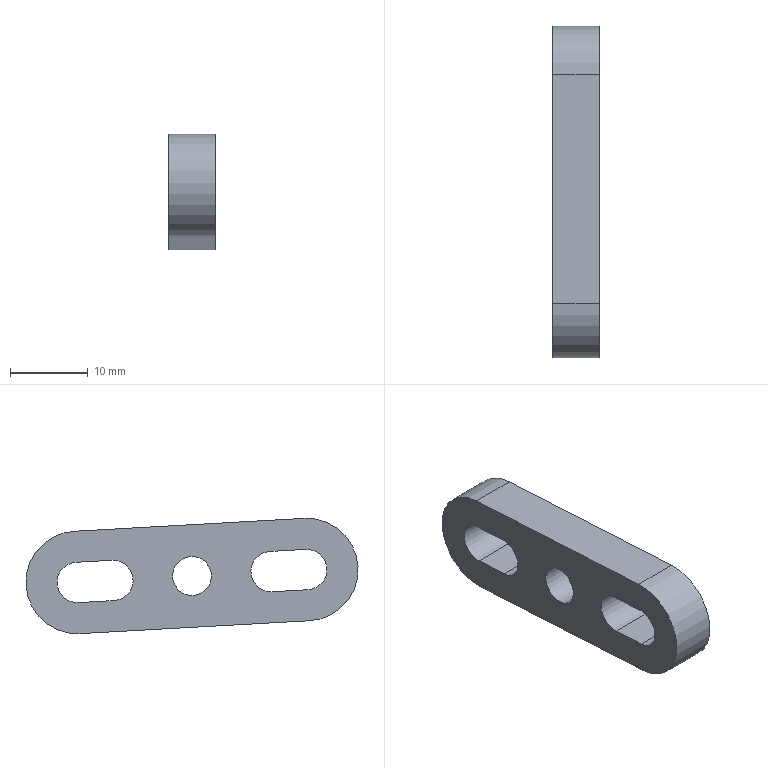Part | STEP file | 1 solid | 15 faces | box 6 x 42.771 x 14.853 mm | volume 2506 mm3 | plane 8 | cylinder 7 | commonest cylinder face diameters 5.2 x4 13.2 x2 5.01 x1
STEP:
#1=CARTESIAN_POINT('',(0.,0.,0.));
#2=DIRECTION('',(0.,0.,1.));
#3=DIRECTION('',(1.,0.,0.));
#4=AXIS2_PLACEMENT_3D('',#1,#2,#3);
#5=CARTESIAN_POINT('',(1826.907,485.05,14.25));
#6=VERTEX_POINT('',#5);
#7=CARTESIAN_POINT('',(1826.907,489.66,13.992));
#8=VERTEX_POINT('',#7);
#9=CARTESIAN_POINT('',(1826.907,489.66,13.992));
#10=DIRECTION('',(0.,0.9984,-0.05582));
#11=VECTOR('',#10,1.);
#12=LINE('',#9,#11);
#13=CARTESIAN_POINT('',(1832.907,489.66,13.992));
#14=DIRECTION('',(0.,0.05582,0.9984));
#15=DIRECTION('',(1.,0.,0.));
#16=AXIS2_PLACEMENT_3D('',#13,#14,#15);
#17=PLANE('',#16);
#18=CARTESIAN_POINT('',(-6.,0.));
#19=DIRECTION('',(0.,1.));
#20=VECTOR('',#19,1.);
#21=LINE('',#18,#20);
#22=(GEOMETRIC_REPRESENTATION_CONTEXT(2)PARAMETRIC_REPRESENTATION_CONTEXT()REPRESENTATION_CONTEXT('',''));
#23=DEFINITIONAL_REPRESENTATION('',(#21),#22);
#24=PCURVE('',#17,#23);
#25=CARTESIAN_POINT('',(1826.907,485.195,16.846));
#26=DIRECTION('',(-1.,0.,0.));
#27=DIRECTION('',(0.,0.05582,0.9984));
#28=AXIS2_PLACEMENT_3D('',#25,#26,#27);
#29=PLANE('',#28);
#30=CARTESIAN_POINT('',(-2.6,4.618));
#31=DIRECTION('',(0.,1.));
#32=VECTOR('',#31,1.);
#33=LINE('',#30,#32);
#34=(GEOMETRIC_REPRESENTATION_CONTEXT(2)PARAMETRIC_REPRESENTATION_CONTEXT()REPRESENTATION_CONTEXT('',''));
#35=DEFINITIONAL_REPRESENTATION('',(#33),#34);
#36=PCURVE('',#29,#35);
#37=SURFACE_CURVE('',#12,(#24,#36),.PCURVE_S1.);
#38=EDGE_CURVE('',#6,#8,#37,.T.);
#39=ORIENTED_EDGE('',*,*,#38,.F.);
#40=CARTESIAN_POINT('',(1832.907,485.05,14.25));
#41=VERTEX_POINT('',#40);
#42=CARTESIAN_POINT('',(1832.907,485.05,14.25));
#43=DIRECTION('',(1.,0.,0.));
#44=VECTOR('',#43,1.);
#45=LINE('',#42,#44);
#46=CARTESIAN_POINT('',(0.,-4.618));
#47=DIRECTION('',(1.,0.));
#48=VECTOR('',#47,1.);
#49=LINE('',#46,#48);
#50=(GEOMETRIC_REPRESENTATION_CONTEXT(2)PARAMETRIC_REPRESENTATION_CONTEXT()REPRESENTATION_CONTEXT('',''));
#51=DEFINITIONAL_REPRESENTATION('',(#49),#50);
#52=PCURVE('',#17,#51);
#53=CARTESIAN_POINT('',(1832.907,485.195,16.846));
#54=DIRECTION('',(-1.,0.,0.));
#55=DIRECTION('',(0.,0.05582,0.9984));
#56=AXIS2_PLACEMENT_3D('',#53,#54,#55);
#57=CYLINDRICAL_SURFACE('',#56,2.6);
#58=CARTESIAN_POINT('',(3.142,0.));
#59=DIRECTION('',(0.,-1.));
#60=VECTOR('',#59,1.);
#61=LINE('',#58,#60);
#62=(GEOMETRIC_REPRESENTATION_CONTEXT(2)PARAMETRIC_REPRESENTATION_CONTEXT()REPRESENTATION_CONTEXT('',''));
#63=DEFINITIONAL_REPRESENTATION('',(#61),#62);
#64=PCURVE('',#57,#63);
#65=SURFACE_CURVE('',#45,(#52,#64),.PCURVE_S1.);
#66=EDGE_CURVE('',#6,#41,#65,.T.);
#67=ORIENTED_EDGE('',*,*,#66,.T.);
#68=CARTESIAN_POINT('',(1832.907,489.66,13.992));
#69=VERTEX_POINT('',#68);
#70=CARTESIAN_POINT('',(1832.907,489.66,13.992));
#71=DIRECTION('',(0.,0.9984,-0.05582));
#72=VECTOR('',#71,1.);
#73=LINE('',#70,#72);
#74=CARTESIAN_POINT('',(0.,0.));
#75=DIRECTION('',(0.,1.));
#76=VECTOR('',#75,1.);
#77=LINE('',#74,#76);
#78=(GEOMETRIC_REPRESENTATION_CONTEXT(2)PARAMETRIC_REPRESENTATION_CONTEXT()REPRESENTATION_CONTEXT('',''));
#79=DEFINITIONAL_REPRESENTATION('',(#77),#78);
#80=PCURVE('',#17,#79);
#81=CARTESIAN_POINT('',(1832.907,485.195,16.846));
#82=DIRECTION('',(-1.,0.,0.));
#83=DIRECTION('',(0.,0.05582,0.9984));
#84=AXIS2_PLACEMENT_3D('',#81,#82,#83);
#85=PLANE('',#84);
#86=CARTESIAN_POINT('',(-2.6,4.618));
#87=DIRECTION('',(0.,1.));
#88=VECTOR('',#87,1.);
#89=LINE('',#86,#88);
#90=(GEOMETRIC_REPRESENTATION_CONTEXT(2)PARAMETRIC_REPRESENTATION_CONTEXT()REPRESENTATION_CONTEXT('',''));
#91=DEFINITIONAL_REPRESENTATION('',(#89),#90);
#92=PCURVE('',#85,#91);
#93=SURFACE_CURVE('',#73,(#80,#92),.PCURVE_S1.);
#94=EDGE_CURVE('',#41,#69,#93,.T.);
#95=ORIENTED_EDGE('',*,*,#94,.T.);
#96=CARTESIAN_POINT('',(1832.907,489.66,13.992));
#97=DIRECTION('',(1.,0.,0.));
#98=VECTOR('',#97,1.);
#99=LINE('',#96,#98);
#100=CARTESIAN_POINT('',(0.,0.));
#101=DIRECTION('',(1.,0.));
#102=VECTOR('',#101,1.);
#103=LINE('',#100,#102);
#104=(GEOMETRIC_REPRESENTATION_CONTEXT(2)PARAMETRIC_REPRESENTATION_CONTEXT()REPRESENTATION_CONTEXT('',''));
#105=DEFINITIONAL_REPRESENTATION('',(#103),#104);
#106=PCURVE('',#17,#105);
#107=CARTESIAN_POINT('',(1832.907,489.805,16.588));
#108=DIRECTION('',(-1.,0.,0.));
#109=DIRECTION('',(0.,0.05582,0.9984));
#110=AXIS2_PLACEMENT_3D('',#107,#108,#109);
#111=CYLINDRICAL_SURFACE('',#110,2.6);
#112=CARTESIAN_POINT('',(3.142,0.));
#113=DIRECTION('',(0.,-1.));
#114=VECTOR('',#113,1.);
#115=LINE('',#112,#114);
#116=(GEOMETRIC_REPRESENTATION_CONTEXT(2)PARAMETRIC_REPRESENTATION_CONTEXT()REPRESENTATION_CONTEXT('',''));
#117=DEFINITIONAL_REPRESENTATION('',(#115),#116);
#118=PCURVE('',#111,#117);
#119=SURFACE_CURVE('',#99,(#106,#118),.PCURVE_S1.);
#120=EDGE_CURVE('',#8,#69,#119,.T.);
#121=ORIENTED_EDGE('',*,*,#120,.F.);
#122=EDGE_LOOP('',(#39,#67,#95,#121));
#123=FACE_BOUND('',#122,.T.);
#124=ADVANCED_FACE('',(#123),#17,.T.);
#125=ORIENTED_EDGE('',*,*,#66,.T.);
#126=CARTESIAN_POINT('',(1832.907,485.34,19.442));
#127=VERTEX_POINT('',#126);
#128=CARTESIAN_POINT('',(1832.907,485.195,16.846));
#129=DIRECTION('',(1.,0.,0.));
#130=DIRECTION('',(0.,0.05582,0.9984));
#131=AXIS2_PLACEMENT_3D('',#128,#129,#130);
#132=CIRCLE('',#131,2.6);
#133=CARTESIAN_POINT('',(6.283,0.));
#134=DIRECTION('',(-1.,0.));
#135=VECTOR('',#134,1.);
#136=LINE('',#133,#135);
#137=(GEOMETRIC_REPRESENTATION_CONTEXT(2)PARAMETRIC_REPRESENTATION_CONTEXT()REPRESENTATION_CONTEXT('',''));
#138=DEFINITIONAL_REPRESENTATION('',(#136),#137);
#139=PCURVE('',#57,#138);
#140=CARTESIAN_POINT('',(2.6,0.));
#141=CARTESIAN_POINT('',(2.6,-4.503));
#142=CARTESIAN_POINT('',(-1.3,-2.252));
#143=CARTESIAN_POINT('',(-5.2,0.));
#144=CARTESIAN_POINT('',(-1.3,2.252));
#145=CARTESIAN_POINT('',(2.6,4.503));
#146=CARTESIAN_POINT('',(2.6,0.));
#147=(BOUNDED_CURVE()B_SPLINE_CURVE(2,(#140,#141,#142,#143,#144,#145,#146),.UNSPECIFIED.,.T.,.F.)B_SPLINE_CURVE_WITH_KNOTS((1,2,2,2,2,1),(-2.094,0.,2.094,4.189,6.283,8.378),.UNSPECIFIED.)CURVE()GEOMETRIC_REPRESENTATION_ITEM()RATIONAL_B_SPLINE_CURVE((1.,0.5,1.,0.5,1.,0.5,1.))REPRESENTATION_ITEM(''));
#148=(GEOMETRIC_REPRESENTATION_CONTEXT(2)PARAMETRIC_REPRESENTATION_CONTEXT()REPRESENTATION_CONTEXT('',''));
#149=DEFINITIONAL_REPRESENTATION('',(#147),#148);
#150=PCURVE('',#85,#149);
#151=SURFACE_CURVE('',#132,(#139,#150),.PCURVE_S1.);
#152=EDGE_CURVE('',#127,#41,#151,.T.);
#153=ORIENTED_EDGE('',*,*,#152,.F.);
#154=CARTESIAN_POINT('',(1826.907,485.34,19.442));
#155=VERTEX_POINT('',#154);
#156=CARTESIAN_POINT('',(1832.907,485.34,19.442));
#157=DIRECTION('',(1.,0.,0.));
#158=VECTOR('',#157,1.);
#159=LINE('',#156,#158);
#160=CARTESIAN_POINT('',(6.283,0.));
#161=DIRECTION('',(0.,-1.));
#162=VECTOR('',#161,1.);
#163=LINE('',#160,#162);
#164=(GEOMETRIC_REPRESENTATION_CONTEXT(2)PARAMETRIC_REPRESENTATION_CONTEXT()REPRESENTATION_CONTEXT('',''));
#165=DEFINITIONAL_REPRESENTATION('',(#163),#164);
#166=PCURVE('',#57,#165);
#167=CARTESIAN_POINT('',(1832.907,485.34,19.442));
#168=DIRECTION('',(0.,-0.05582,-0.9984));
#169=DIRECTION('',(-1.,0.,0.));
#170=AXIS2_PLACEMENT_3D('',#167,#168,#169);
#171=PLANE('',#170);
#172=CARTESIAN_POINT('',(0.,0.));
#173=DIRECTION('',(-1.,0.));
#174=VECTOR('',#173,1.);
#175=LINE('',#172,#174);
#176=(GEOMETRIC_REPRESENTATION_CONTEXT(2)PARAMETRIC_REPRESENTATION_CONTEXT()REPRESENTATION_CONTEXT('',''));
#177=DEFINITIONAL_REPRESENTATION('',(#175),#176);
#178=PCURVE('',#171,#177);
#179=SURFACE_CURVE('',#159,(#166,#178),.PCURVE_S1.);
#180=EDGE_CURVE('',#155,#127,#179,.T.);
#181=ORIENTED_EDGE('',*,*,#180,.F.);
#182=CARTESIAN_POINT('',(1826.907,485.195,16.846));
#183=DIRECTION('',(1.,0.,0.));
#184=DIRECTION('',(0.,0.05582,0.9984));
#185=AXIS2_PLACEMENT_3D('',#182,#183,#184);
#186=CIRCLE('',#185,2.6);
#187=CARTESIAN_POINT('',(6.283,6.));
#188=DIRECTION('',(-1.,0.));
#189=VECTOR('',#188,1.);
#190=LINE('',#187,#189);
#191=(GEOMETRIC_REPRESENTATION_CONTEXT(2)PARAMETRIC_REPRESENTATION_CONTEXT()REPRESENTATION_CONTEXT('',''));
#192=DEFINITIONAL_REPRESENTATION('',(#190),#191);
#193=PCURVE('',#57,#192);
#194=CARTESIAN_POINT('',(2.6,0.));
#195=CARTESIAN_POINT('',(2.6,-4.503));
#196=CARTESIAN_POINT('',(-1.3,-2.252));
#197=CARTESIAN_POINT('',(-5.2,0.));
#198=CARTESIAN_POINT('',(-1.3,2.252));
#199=CARTESIAN_POINT('',(2.6,4.503));
#200=CARTESIAN_POINT('',(2.6,0.));
#201=(BOUNDED_CURVE()B_SPLINE_CURVE(2,(#194,#195,#196,#197,#198,#199,#200),.UNSPECIFIED.,.T.,.F.)B_SPLINE_CURVE_WITH_KNOTS((1,2,2,2,2,1),(-2.094,0.,2.094,4.189,6.283,8.378),.UNSPECIFIED.)CURVE()GEOMETRIC_REPRESENTATION_ITEM()RATIONAL_B_SPLINE_CURVE((1.,0.5,1.,0.5,1.,0.5,1.))REPRESENTATION_ITEM(''));
#202=(GEOMETRIC_REPRESENTATION_CONTEXT(2)PARAMETRIC_REPRESENTATION_CONTEXT()REPRESENTATION_CONTEXT('',''));
#203=DEFINITIONAL_REPRESENTATION('',(#201),#202);
#204=PCURVE('',#29,#203);
#205=SURFACE_CURVE('',#186,(#193,#204),.PCURVE_S1.);
#206=EDGE_CURVE('',#155,#6,#205,.T.);
#207=ORIENTED_EDGE('',*,*,#206,.T.);
#208=EDGE_LOOP('',(#125,#153,#181,#207));
#209=FACE_BOUND('',#208,.F.);
#210=ADVANCED_FACE('',(#209),#57,.F.);
#211=CARTESIAN_POINT('',(1826.907,489.95,19.184));
#212=VERTEX_POINT('',#211);
#213=CARTESIAN_POINT('',(1826.907,485.34,19.442));
#214=DIRECTION('',(0.,-0.9984,0.05582));
#215=VECTOR('',#214,1.);
#216=LINE('',#213,#215);
#217=CARTESIAN_POINT('',(6.,0.));
#218=DIRECTION('',(0.,-1.));
#219=VECTOR('',#218,1.);
#220=LINE('',#217,#219);
#221=(GEOMETRIC_REPRESENTATION_CONTEXT(2)PARAMETRIC_REPRESENTATION_CONTEXT()REPRESENTATION_CONTEXT('',''));
#222=DEFINITIONAL_REPRESENTATION('',(#220),#221);
#223=PCURVE('',#171,#222);
#224=CARTESIAN_POINT('',(2.6,0.));
#225=DIRECTION('',(0.,-1.));
#226=VECTOR('',#225,1.);
#227=LINE('',#224,#226);
#228=(GEOMETRIC_REPRESENTATION_CONTEXT(2)PARAMETRIC_REPRESENTATION_CONTEXT()REPRESENTATION_CONTEXT('',''));
#229=DEFINITIONAL_REPRESENTATION('',(#227),#228);
#230=PCURVE('',#29,#229);
#231=SURFACE_CURVE('',#216,(#223,#230),.PCURVE_S1.);
#232=EDGE_CURVE('',#212,#155,#231,.T.);
#233=ORIENTED_EDGE('',*,*,#232,.F.);
#234=CARTESIAN_POINT('',(1832.907,489.95,19.184));
#235=VERTEX_POINT('',#234);
#236=CARTESIAN_POINT('',(1832.907,489.95,19.184));
#237=DIRECTION('',(1.,0.,0.));
#238=VECTOR('',#237,1.);
#239=LINE('',#236,#238);
#240=CARTESIAN_POINT('',(0.,4.618));
#241=DIRECTION('',(-1.,0.));
#242=VECTOR('',#241,1.);
#243=LINE('',#240,#242);
#244=(GEOMETRIC_REPRESENTATION_CONTEXT(2)PARAMETRIC_REPRESENTATION_CONTEXT()REPRESENTATION_CONTEXT('',''));
#245=DEFINITIONAL_REPRESENTATION('',(#243),#244);
#246=PCURVE('',#171,#245);
#247=CARTESIAN_POINT('',(0.,0.));
#248=DIRECTION('',(0.,-1.));
#249=VECTOR('',#248,1.);
#250=LINE('',#247,#249);
#251=(GEOMETRIC_REPRESENTATION_CONTEXT(2)PARAMETRIC_REPRESENTATION_CONTEXT()REPRESENTATION_CONTEXT('',''));
#252=DEFINITIONAL_REPRESENTATION('',(#250),#251);
#253=PCURVE('',#111,#252);
#254=SURFACE_CURVE('',#239,(#246,#253),.PCURVE_S1.);
#255=EDGE_CURVE('',#212,#235,#254,.T.);
#256=ORIENTED_EDGE('',*,*,#255,.T.);
#257=CARTESIAN_POINT('',(1832.907,485.34,19.442));
#258=DIRECTION('',(0.,-0.9984,0.05582));
#259=VECTOR('',#258,1.);
#260=LINE('',#257,#259);
#261=CARTESIAN_POINT('',(0.,0.));
#262=DIRECTION('',(0.,-1.));
#263=VECTOR('',#262,1.);
#264=LINE('',#261,#263);
#265=(GEOMETRIC_REPRESENTATION_CONTEXT(2)PARAMETRIC_REPRESENTATION_CONTEXT()REPRESENTATION_CONTEXT('',''));
#266=DEFINITIONAL_REPRESENTATION('',(#264),#265);
#267=PCURVE('',#171,#266);
#268=CARTESIAN_POINT('',(2.6,0.));
#269=DIRECTION('',(0.,-1.));
#270=VECTOR('',#269,1.);
#271=LINE('',#268,#270);
#272=(GEOMETRIC_REPRESENTATION_CONTEXT(2)PARAMETRIC_REPRESENTATION_CONTEXT()REPRESENTATION_CONTEXT('',''));
#273=DEFINITIONAL_REPRESENTATION('',(#271),#272);
#274=PCURVE('',#85,#273);
#275=SURFACE_CURVE('',#260,(#267,#274),.PCURVE_S1.);
#276=EDGE_CURVE('',#235,#127,#275,.T.);
#277=ORIENTED_EDGE('',*,*,#276,.T.);
#278=ORIENTED_EDGE('',*,*,#180,.F.);
#279=EDGE_LOOP('',(#233,#256,#277,#278));
#280=FACE_BOUND('',#279,.T.);
#281=ADVANCED_FACE('',(#280),#171,.T.);
#282=CARTESIAN_POINT('',(1826.907,510.01,12.854));
#283=VERTEX_POINT('',#282);
#284=CARTESIAN_POINT('',(1826.907,514.621,12.597));
#285=VERTEX_POINT('',#284);
#286=CARTESIAN_POINT('',(1826.907,514.621,12.597));
#287=DIRECTION('',(0.,0.9984,-0.05582));
#288=VECTOR('',#287,1.);
#289=LINE('',#286,#288);
#290=CARTESIAN_POINT('',(1832.907,514.621,12.597));
#291=DIRECTION('',(0.,0.05582,0.9984));
#292=DIRECTION('',(0.,-0.9984,0.05582));
#293=AXIS2_PLACEMENT_3D('',#290,#291,#292);
#294=PLANE('',#293);
#295=CARTESIAN_POINT('',(0.,-6.));
#296=DIRECTION('',(-1.,0.));
#297=VECTOR('',#296,1.);
#298=LINE('',#295,#297);
#299=(GEOMETRIC_REPRESENTATION_CONTEXT(2)PARAMETRIC_REPRESENTATION_CONTEXT()REPRESENTATION_CONTEXT('',''));
#300=DEFINITIONAL_REPRESENTATION('',(#298),#299);
#301=PCURVE('',#294,#300);
#302=CARTESIAN_POINT('',(-2.6,29.617));
#303=DIRECTION('',(0.,1.));
#304=VECTOR('',#303,1.);
#305=LINE('',#302,#304);
#306=(GEOMETRIC_REPRESENTATION_CONTEXT(2)PARAMETRIC_REPRESENTATION_CONTEXT()REPRESENTATION_CONTEXT('',''));
#307=DEFINITIONAL_REPRESENTATION('',(#305),#306);
#308=PCURVE('',#29,#307);
#309=SURFACE_CURVE('',#289,(#301,#308),.PCURVE_S1.);
#310=EDGE_CURVE('',#283,#285,#309,.T.);
#311=ORIENTED_EDGE('',*,*,#310,.F.);
#312=CARTESIAN_POINT('',(1832.907,510.01,12.854));
#313=VERTEX_POINT('',#312);
#314=CARTESIAN_POINT('',(1832.907,510.01,12.854));
#315=DIRECTION('',(1.,0.,0.));
#316=VECTOR('',#315,1.);
#317=LINE('',#314,#316);
#318=CARTESIAN_POINT('',(4.618,0.));
#319=DIRECTION('',(0.,1.));
#320=VECTOR('',#319,1.);
#321=LINE('',#318,#320);
#322=(GEOMETRIC_REPRESENTATION_CONTEXT(2)PARAMETRIC_REPRESENTATION_CONTEXT()REPRESENTATION_CONTEXT('',''));
#323=DEFINITIONAL_REPRESENTATION('',(#321),#322);
#324=PCURVE('',#294,#323);
#325=CARTESIAN_POINT('',(1832.907,510.156,15.45));
#326=DIRECTION('',(-1.,0.,0.));
#327=DIRECTION('',(0.,0.05582,0.9984));
#328=AXIS2_PLACEMENT_3D('',#325,#326,#327);
#329=CYLINDRICAL_SURFACE('',#328,2.6);
#330=CARTESIAN_POINT('',(3.142,0.));
#331=DIRECTION('',(0.,-1.));
#332=VECTOR('',#331,1.);
#333=LINE('',#330,#332);
#334=(GEOMETRIC_REPRESENTATION_CONTEXT(2)PARAMETRIC_REPRESENTATION_CONTEXT()REPRESENTATION_CONTEXT('',''));
#335=DEFINITIONAL_REPRESENTATION('',(#333),#334);
#336=PCURVE('',#329,#335);
#337=SURFACE_CURVE('',#317,(#324,#336),.PCURVE_S1.);
#338=EDGE_CURVE('',#283,#313,#337,.T.);
#339=ORIENTED_EDGE('',*,*,#338,.T.);
#340=CARTESIAN_POINT('',(1832.907,514.621,12.597));
#341=VERTEX_POINT('',#340);
#342=CARTESIAN_POINT('',(1832.907,514.621,12.597));
#343=DIRECTION('',(0.,0.9984,-0.05582));
#344=VECTOR('',#343,1.);
#345=LINE('',#342,#344);
#346=CARTESIAN_POINT('',(0.,0.));
#347=DIRECTION('',(-1.,0.));
#348=VECTOR('',#347,1.);
#349=LINE('',#346,#348);
#350=(GEOMETRIC_REPRESENTATION_CONTEXT(2)PARAMETRIC_REPRESENTATION_CONTEXT()REPRESENTATION_CONTEXT('',''));
#351=DEFINITIONAL_REPRESENTATION('',(#349),#350);
#352=PCURVE('',#294,#351);
#353=CARTESIAN_POINT('',(-2.6,29.617));
#354=DIRECTION('',(0.,1.));
#355=VECTOR('',#354,1.);
#356=LINE('',#353,#355);
#357=(GEOMETRIC_REPRESENTATION_CONTEXT(2)PARAMETRIC_REPRESENTATION_CONTEXT()REPRESENTATION_CONTEXT('',''));
#358=DEFINITIONAL_REPRESENTATION('',(#356),#357);
#359=PCURVE('',#85,#358);
#360=SURFACE_CURVE('',#345,(#352,#359),.PCURVE_S1.);
#361=EDGE_CURVE('',#313,#341,#360,.T.);
#362=ORIENTED_EDGE('',*,*,#361,.T.);
#363=CARTESIAN_POINT('',(1832.907,514.621,12.597));
#364=DIRECTION('',(1.,0.,0.));
#365=VECTOR('',#364,1.);
#366=LINE('',#363,#365);
#367=CARTESIAN_POINT('',(0.,0.));
#368=DIRECTION('',(0.,1.));
#369=VECTOR('',#368,1.);
#370=LINE('',#367,#369);
#371=(GEOMETRIC_REPRESENTATION_CONTEXT(2)PARAMETRIC_REPRESENTATION_CONTEXT()REPRESENTATION_CONTEXT('',''));
#372=DEFINITIONAL_REPRESENTATION('',(#370),#371);
#373=PCURVE('',#294,#372);
#374=CARTESIAN_POINT('',(1832.907,514.766,15.192));
#375=DIRECTION('',(-1.,0.,0.));
#376=DIRECTION('',(0.,0.05582,0.9984));
#377=AXIS2_PLACEMENT_3D('',#374,#375,#376);
#378=CYLINDRICAL_SURFACE('',#377,2.6);
#379=CARTESIAN_POINT('',(3.142,0.));
#380=DIRECTION('',(0.,-1.));
#381=VECTOR('',#380,1.);
#382=LINE('',#379,#381);
#383=(GEOMETRIC_REPRESENTATION_CONTEXT(2)PARAMETRIC_REPRESENTATION_CONTEXT()REPRESENTATION_CONTEXT('',''));
#384=DEFINITIONAL_REPRESENTATION('',(#382),#383);
#385=PCURVE('',#378,#384);
#386=SURFACE_CURVE('',#366,(#373,#385),.PCURVE_S1.);
#387=EDGE_CURVE('',#285,#341,#386,.T.);
#388=ORIENTED_EDGE('',*,*,#387,.F.);
#389=EDGE_LOOP('',(#311,#339,#362,#388));
#390=FACE_BOUND('',#389,.T.);
#391=ADVANCED_FACE('',(#390),#294,.T.);
#392=ORIENTED_EDGE('',*,*,#338,.T.);
#393=CARTESIAN_POINT('',(1832.907,510.301,18.046));
#394=VERTEX_POINT('',#393);
#395=CARTESIAN_POINT('',(1832.907,510.156,15.45));
#396=DIRECTION('',(1.,0.,0.));
#397=DIRECTION('',(0.,0.05582,0.9984));
#398=AXIS2_PLACEMENT_3D('',#395,#396,#397);
#399=CIRCLE('',#398,2.6);
#400=CARTESIAN_POINT('',(6.283,0.));
#401=DIRECTION('',(-1.,0.));
#402=VECTOR('',#401,1.);
#403=LINE('',#400,#402);
#404=(GEOMETRIC_REPRESENTATION_CONTEXT(2)PARAMETRIC_REPRESENTATION_CONTEXT()REPRESENTATION_CONTEXT('',''));
#405=DEFINITIONAL_REPRESENTATION('',(#403),#404);
#406=PCURVE('',#329,#405);
#407=CARTESIAN_POINT('',(2.6,25.));
#408=CARTESIAN_POINT('',(2.6,20.496));
#409=CARTESIAN_POINT('',(-1.3,22.748));
#410=CARTESIAN_POINT('',(-5.2,25.));
#411=CARTESIAN_POINT('',(-1.3,27.251));
#412=CARTESIAN_POINT('',(2.6,29.503));
#413=CARTESIAN_POINT('',(2.6,25.));
#414=(BOUNDED_CURVE()B_SPLINE_CURVE(2,(#407,#408,#409,#410,#411,#412,#413),.UNSPECIFIED.,.T.,.F.)B_SPLINE_CURVE_WITH_KNOTS((1,2,2,2,2,1),(-2.094,0.,2.094,4.189,6.283,8.378),.UNSPECIFIED.)CURVE()GEOMETRIC_REPRESENTATION_ITEM()RATIONAL_B_SPLINE_CURVE((1.,0.5,1.,0.5,1.,0.5,1.))REPRESENTATION_ITEM(''));
#415=(GEOMETRIC_REPRESENTATION_CONTEXT(2)PARAMETRIC_REPRESENTATION_CONTEXT()REPRESENTATION_CONTEXT('',''));
#416=DEFINITIONAL_REPRESENTATION('',(#414),#415);
#417=PCURVE('',#85,#416);
#418=SURFACE_CURVE('',#399,(#406,#417),.PCURVE_S1.);
#419=EDGE_CURVE('',#394,#313,#418,.T.);
#420=ORIENTED_EDGE('',*,*,#419,.F.);
#421=CARTESIAN_POINT('',(1826.907,510.301,18.046));
#422=VERTEX_POINT('',#421);
#423=CARTESIAN_POINT('',(1832.907,510.301,18.046));
#424=DIRECTION('',(1.,0.,0.));
#425=VECTOR('',#424,1.);
#426=LINE('',#423,#425);
#427=CARTESIAN_POINT('',(6.283,0.));
#428=DIRECTION('',(0.,-1.));
#429=VECTOR('',#428,1.);
#430=LINE('',#427,#429);
#431=(GEOMETRIC_REPRESENTATION_CONTEXT(2)PARAMETRIC_REPRESENTATION_CONTEXT()REPRESENTATION_CONTEXT('',''));
#432=DEFINITIONAL_REPRESENTATION('',(#430),#431);
#433=PCURVE('',#329,#432);
#434=CARTESIAN_POINT('',(1832.907,510.301,18.046));
#435=DIRECTION('',(0.,-0.05582,-0.9984));
#436=DIRECTION('',(-1.,0.,0.));
#437=AXIS2_PLACEMENT_3D('',#434,#435,#436);
#438=PLANE('',#437);
#439=CARTESIAN_POINT('',(0.,0.));
#440=DIRECTION('',(-1.,0.));
#441=VECTOR('',#440,1.);
#442=LINE('',#439,#441);
#443=(GEOMETRIC_REPRESENTATION_CONTEXT(2)PARAMETRIC_REPRESENTATION_CONTEXT()REPRESENTATION_CONTEXT('',''));
#444=DEFINITIONAL_REPRESENTATION('',(#442),#443);
#445=PCURVE('',#438,#444);
#446=SURFACE_CURVE('',#426,(#433,#445),.PCURVE_S1.);
#447=EDGE_CURVE('',#422,#394,#446,.T.);
#448=ORIENTED_EDGE('',*,*,#447,.F.);
#449=CARTESIAN_POINT('',(1826.907,510.156,15.45));
#450=DIRECTION('',(1.,0.,0.));
#451=DIRECTION('',(0.,0.05582,0.9984));
#452=AXIS2_PLACEMENT_3D('',#449,#450,#451);
#453=CIRCLE('',#452,2.6);
#454=CARTESIAN_POINT('',(6.283,6.));
#455=DIRECTION('',(-1.,0.));
#456=VECTOR('',#455,1.);
#457=LINE('',#454,#456);
#458=(GEOMETRIC_REPRESENTATION_CONTEXT(2)PARAMETRIC_REPRESENTATION_CONTEXT()REPRESENTATION_CONTEXT('',''));
#459=DEFINITIONAL_REPRESENTATION('',(#457),#458);
#460=PCURVE('',#329,#459);
#461=CARTESIAN_POINT('',(2.6,25.));
#462=CARTESIAN_POINT('',(2.6,20.496));
#463=CARTESIAN_POINT('',(-1.3,22.748));
#464=CARTESIAN_POINT('',(-5.2,25.));
#465=CARTESIAN_POINT('',(-1.3,27.251));
#466=CARTESIAN_POINT('',(2.6,29.503));
#467=CARTESIAN_POINT('',(2.6,25.));
#468=(BOUNDED_CURVE()B_SPLINE_CURVE(2,(#461,#462,#463,#464,#465,#466,#467),.UNSPECIFIED.,.T.,.F.)B_SPLINE_CURVE_WITH_KNOTS((1,2,2,2,2,1),(-2.094,0.,2.094,4.189,6.283,8.378),.UNSPECIFIED.)CURVE()GEOMETRIC_REPRESENTATION_ITEM()RATIONAL_B_SPLINE_CURVE((1.,0.5,1.,0.5,1.,0.5,1.))REPRESENTATION_ITEM(''));
#469=(GEOMETRIC_REPRESENTATION_CONTEXT(2)PARAMETRIC_REPRESENTATION_CONTEXT()REPRESENTATION_CONTEXT('',''));
#470=DEFINITIONAL_REPRESENTATION('',(#468),#469);
#471=PCURVE('',#29,#470);
#472=SURFACE_CURVE('',#453,(#460,#471),.PCURVE_S1.);
#473=EDGE_CURVE('',#422,#283,#472,.T.);
#474=ORIENTED_EDGE('',*,*,#473,.T.);
#475=EDGE_LOOP('',(#392,#420,#448,#474));
#476=FACE_BOUND('',#475,.F.);
#477=ADVANCED_FACE('',(#476),#329,.F.);
#478=CARTESIAN_POINT('',(1826.907,514.911,17.788));
#479=VERTEX_POINT('',#478);
#480=CARTESIAN_POINT('',(1826.907,510.301,18.046));
#481=DIRECTION('',(0.,-0.9984,0.05582));
#482=VECTOR('',#481,1.);
#483=LINE('',#480,#482);
#484=CARTESIAN_POINT('',(6.,0.));
#485=DIRECTION('',(0.,-1.));
#486=VECTOR('',#485,1.);
#487=LINE('',#484,#486);
#488=(GEOMETRIC_REPRESENTATION_CONTEXT(2)PARAMETRIC_REPRESENTATION_CONTEXT()REPRESENTATION_CONTEXT('',''));
#489=DEFINITIONAL_REPRESENTATION('',(#487),#488);
#490=PCURVE('',#438,#489);
#491=CARTESIAN_POINT('',(2.6,25.));
#492=DIRECTION('',(0.,-1.));
#493=VECTOR('',#492,1.);
#494=LINE('',#491,#493);
#495=(GEOMETRIC_REPRESENTATION_CONTEXT(2)PARAMETRIC_REPRESENTATION_CONTEXT()REPRESENTATION_CONTEXT('',''));
#496=DEFINITIONAL_REPRESENTATION('',(#494),#495);
#497=PCURVE('',#29,#496);
#498=SURFACE_CURVE('',#483,(#490,#497),.PCURVE_S1.);
#499=EDGE_CURVE('',#479,#422,#498,.T.);
#500=ORIENTED_EDGE('',*,*,#499,.F.);
#501=CARTESIAN_POINT('',(1832.907,514.911,17.788));
#502=VERTEX_POINT('',#501);
#503=CARTESIAN_POINT('',(1832.907,514.911,17.788));
#504=DIRECTION('',(1.,0.,0.));
#505=VECTOR('',#504,1.);
#506=LINE('',#503,#505);
#507=CARTESIAN_POINT('',(0.,4.618));
#508=DIRECTION('',(-1.,0.));
#509=VECTOR('',#508,1.);
#510=LINE('',#507,#509);
#511=(GEOMETRIC_REPRESENTATION_CONTEXT(2)PARAMETRIC_REPRESENTATION_CONTEXT()REPRESENTATION_CONTEXT('',''));
#512=DEFINITIONAL_REPRESENTATION('',(#510),#511);
#513=PCURVE('',#438,#512);
#514=CARTESIAN_POINT('',(0.,0.));
#515=DIRECTION('',(0.,-1.));
#516=VECTOR('',#515,1.);
#517=LINE('',#514,#516);
#518=(GEOMETRIC_REPRESENTATION_CONTEXT(2)PARAMETRIC_REPRESENTATION_CONTEXT()REPRESENTATION_CONTEXT('',''));
#519=DEFINITIONAL_REPRESENTATION('',(#517),#518);
#520=PCURVE('',#378,#519);
#521=SURFACE_CURVE('',#506,(#513,#520),.PCURVE_S1.);
#522=EDGE_CURVE('',#479,#502,#521,.T.);
#523=ORIENTED_EDGE('',*,*,#522,.T.);
#524=CARTESIAN_POINT('',(1832.907,510.301,18.046));
#525=DIRECTION('',(0.,-0.9984,0.05582));
#526=VECTOR('',#525,1.);
#527=LINE('',#524,#526);
#528=CARTESIAN_POINT('',(0.,0.));
#529=DIRECTION('',(0.,-1.));
#530=VECTOR('',#529,1.);
#531=LINE('',#528,#530);
#532=(GEOMETRIC_REPRESENTATION_CONTEXT(2)PARAMETRIC_REPRESENTATION_CONTEXT()REPRESENTATION_CONTEXT('',''));
#533=DEFINITIONAL_REPRESENTATION('',(#531),#532);
#534=PCURVE('',#438,#533);
#535=CARTESIAN_POINT('',(2.6,25.));
#536=DIRECTION('',(0.,-1.));
#537=VECTOR('',#536,1.);
#538=LINE('',#535,#537);
#539=(GEOMETRIC_REPRESENTATION_CONTEXT(2)PARAMETRIC_REPRESENTATION_CONTEXT()REPRESENTATION_CONTEXT('',''));
#540=DEFINITIONAL_REPRESENTATION('',(#538),#539);
#541=PCURVE('',#85,#540);
#542=SURFACE_CURVE('',#527,(#534,#541),.PCURVE_S1.);
#543=EDGE_CURVE('',#502,#394,#542,.T.);
#544=ORIENTED_EDGE('',*,*,#543,.T.);
#545=ORIENTED_EDGE('',*,*,#447,.F.);
#546=EDGE_LOOP('',(#500,#523,#544,#545));
#547=FACE_BOUND('',#546,.T.);
#548=ADVANCED_FACE('',(#547),#438,.T.);
#549=CARTESIAN_POINT('',(1826.907,485.563,23.435));
#550=VERTEX_POINT('',#549);
#551=CARTESIAN_POINT('',(1826.907,515.135,21.782));
#552=VERTEX_POINT('',#551);
#553=CARTESIAN_POINT('',(1826.907,515.135,21.782));
#554=DIRECTION('',(0.,0.9984,-0.05582));
#555=VECTOR('',#554,1.);
#556=LINE('',#553,#555);
#557=CARTESIAN_POINT('',(1832.907,515.135,21.782));
#558=DIRECTION('',(0.,0.05582,0.9984));
#559=DIRECTION('',(0.,-0.9984,0.05582));
#560=AXIS2_PLACEMENT_3D('',#557,#558,#559);
#561=PLANE('',#560);
#562=CARTESIAN_POINT('',(0.,-6.));
#563=DIRECTION('',(-1.,0.));
#564=VECTOR('',#563,1.);
#565=LINE('',#562,#564);
#566=(GEOMETRIC_REPRESENTATION_CONTEXT(2)PARAMETRIC_REPRESENTATION_CONTEXT()REPRESENTATION_CONTEXT('',''));
#567=DEFINITIONAL_REPRESENTATION('',(#565),#566);
#568=PCURVE('',#561,#567);
#569=CARTESIAN_POINT('',(6.6,29.617));
#570=DIRECTION('',(0.,1.));
#571=VECTOR('',#570,1.);
#572=LINE('',#569,#571);
#573=(GEOMETRIC_REPRESENTATION_CONTEXT(2)PARAMETRIC_REPRESENTATION_CONTEXT()REPRESENTATION_CONTEXT('',''));
#574=DEFINITIONAL_REPRESENTATION('',(#572),#573);
#575=PCURVE('',#29,#574);
#576=SURFACE_CURVE('',#556,(#568,#575),.PCURVE_S1.);
#577=EDGE_CURVE('',#550,#552,#576,.T.);
#578=ORIENTED_EDGE('',*,*,#577,.F.);
#579=CARTESIAN_POINT('',(1832.907,485.563,23.435));
#580=VERTEX_POINT('',#579);
#581=CARTESIAN_POINT('',(1832.907,485.563,23.435));
#582=DIRECTION('',(1.,0.,0.));
#583=VECTOR('',#582,1.);
#584=LINE('',#581,#583);
#585=CARTESIAN_POINT('',(29.617,0.));
#586=DIRECTION('',(0.,1.));
#587=VECTOR('',#586,1.);
#588=LINE('',#585,#587);
#589=(GEOMETRIC_REPRESENTATION_CONTEXT(2)PARAMETRIC_REPRESENTATION_CONTEXT()REPRESENTATION_CONTEXT('',''));
#590=DEFINITIONAL_REPRESENTATION('',(#588),#589);
#591=PCURVE('',#561,#590);
#592=CARTESIAN_POINT('',(1832.907,485.195,16.846));
#593=DIRECTION('',(-1.,0.,0.));
#594=DIRECTION('',(0.,0.05582,0.9984));
#595=AXIS2_PLACEMENT_3D('',#592,#593,#594);
#596=CYLINDRICAL_SURFACE('',#595,6.6);
#597=CARTESIAN_POINT('',(6.283,0.));
#598=DIRECTION('',(0.,-1.));
#599=VECTOR('',#598,1.);
#600=LINE('',#597,#599);
#601=(GEOMETRIC_REPRESENTATION_CONTEXT(2)PARAMETRIC_REPRESENTATION_CONTEXT()REPRESENTATION_CONTEXT('',''));
#602=DEFINITIONAL_REPRESENTATION('',(#600),#601);
#603=PCURVE('',#596,#602);
#604=SURFACE_CURVE('',#584,(#591,#603),.PCURVE_S1.);
#605=EDGE_CURVE('',#550,#580,#604,.T.);
#606=ORIENTED_EDGE('',*,*,#605,.T.);
#607=CARTESIAN_POINT('',(1832.907,515.135,21.782));
#608=VERTEX_POINT('',#607);
#609=CARTESIAN_POINT('',(1832.907,515.135,21.782));
#610=DIRECTION('',(0.,0.9984,-0.05582));
#611=VECTOR('',#610,1.);
#612=LINE('',#609,#611);
#613=CARTESIAN_POINT('',(0.,0.));
#614=DIRECTION('',(-1.,0.));
#615=VECTOR('',#614,1.);
#616=LINE('',#613,#615);
#617=(GEOMETRIC_REPRESENTATION_CONTEXT(2)PARAMETRIC_REPRESENTATION_CONTEXT()REPRESENTATION_CONTEXT('',''));
#618=DEFINITIONAL_REPRESENTATION('',(#616),#617);
#619=PCURVE('',#561,#618);
#620=CARTESIAN_POINT('',(6.6,29.617));
#621=DIRECTION('',(0.,1.));
#622=VECTOR('',#621,1.);
#623=LINE('',#620,#622);
#624=(GEOMETRIC_REPRESENTATION_CONTEXT(2)PARAMETRIC_REPRESENTATION_CONTEXT()REPRESENTATION_CONTEXT('',''));
#625=DEFINITIONAL_REPRESENTATION('',(#623),#624);
#626=PCURVE('',#85,#625);
#627=SURFACE_CURVE('',#612,(#619,#626),.PCURVE_S1.);
#628=EDGE_CURVE('',#580,#608,#627,.T.);
#629=ORIENTED_EDGE('',*,*,#628,.T.);
#630=CARTESIAN_POINT('',(1832.907,515.135,21.782));
#631=DIRECTION('',(1.,0.,0.));
#632=VECTOR('',#631,1.);
#633=LINE('',#630,#632);
#634=CARTESIAN_POINT('',(0.,0.));
#635=DIRECTION('',(0.,1.));
#636=VECTOR('',#635,1.);
#637=LINE('',#634,#636);
#638=(GEOMETRIC_REPRESENTATION_CONTEXT(2)PARAMETRIC_REPRESENTATION_CONTEXT()REPRESENTATION_CONTEXT('',''));
#639=DEFINITIONAL_REPRESENTATION('',(#637),#638);
#640=PCURVE('',#561,#639);
#641=CARTESIAN_POINT('',(1832.907,514.766,15.192));
#642=DIRECTION('',(-1.,0.,0.));
#643=DIRECTION('',(0.,0.05582,0.9984));
#644=AXIS2_PLACEMENT_3D('',#641,#642,#643);
#645=CYLINDRICAL_SURFACE('',#644,6.6);
#646=CARTESIAN_POINT('',(0.,0.));
#647=DIRECTION('',(0.,-1.));
#648=VECTOR('',#647,1.);
#649=LINE('',#646,#648);
#650=(GEOMETRIC_REPRESENTATION_CONTEXT(2)PARAMETRIC_REPRESENTATION_CONTEXT()REPRESENTATION_CONTEXT('',''));
#651=DEFINITIONAL_REPRESENTATION('',(#649),#650);
#652=PCURVE('',#645,#651);
#653=SURFACE_CURVE('',#633,(#640,#652),.PCURVE_S1.);
#654=EDGE_CURVE('',#552,#608,#653,.T.);
#655=ORIENTED_EDGE('',*,*,#654,.F.);
#656=EDGE_LOOP('',(#578,#606,#629,#655));
#657=FACE_BOUND('',#656,.T.);
#658=ADVANCED_FACE('',(#657),#561,.T.);
#659=CARTESIAN_POINT('',(1826.907,484.826,10.256));
#660=VERTEX_POINT('',#659);
#661=CARTESIAN_POINT('',(1826.907,485.195,16.846));
#662=DIRECTION('',(-1.,0.,0.));
#663=DIRECTION('',(0.,0.05582,0.9984));
#664=AXIS2_PLACEMENT_3D('',#661,#662,#663);
#665=CIRCLE('',#664,6.6);
#666=CARTESIAN_POINT('',(0.,6.));
#667=DIRECTION('',(1.,0.));
#668=VECTOR('',#667,1.);
#669=LINE('',#666,#668);
#670=(GEOMETRIC_REPRESENTATION_CONTEXT(2)PARAMETRIC_REPRESENTATION_CONTEXT()REPRESENTATION_CONTEXT('',''));
#671=DEFINITIONAL_REPRESENTATION('',(#669),#670);
#672=PCURVE('',#596,#671);
#673=CARTESIAN_POINT('',(0.,0.));
#674=DIRECTION('',(1.,0.));
#675=AXIS2_PLACEMENT_2D('',#673,#674);
#676=CIRCLE('',#675,6.6);
#677=(GEOMETRIC_REPRESENTATION_CONTEXT(2)PARAMETRIC_REPRESENTATION_CONTEXT()REPRESENTATION_CONTEXT('',''));
#678=DEFINITIONAL_REPRESENTATION('',(#676),#677);
#679=PCURVE('',#29,#678);
#680=SURFACE_CURVE('',#665,(#672,#679),.PCURVE_S1.);
#681=EDGE_CURVE('',#660,#550,#680,.T.);
#682=ORIENTED_EDGE('',*,*,#681,.F.);
#683=CARTESIAN_POINT('',(1832.907,484.826,10.256));
#684=VERTEX_POINT('',#683);
#685=CARTESIAN_POINT('',(1832.907,484.826,10.256));
#686=DIRECTION('',(1.,0.,0.));
#687=VECTOR('',#686,1.);
#688=LINE('',#685,#687);
#689=CARTESIAN_POINT('',(3.142,0.));
#690=DIRECTION('',(0.,-1.));
#691=VECTOR('',#690,1.);
#692=LINE('',#689,#691);
#693=(GEOMETRIC_REPRESENTATION_CONTEXT(2)PARAMETRIC_REPRESENTATION_CONTEXT()REPRESENTATION_CONTEXT('',''));
#694=DEFINITIONAL_REPRESENTATION('',(#692),#693);
#695=PCURVE('',#596,#694);
#696=CARTESIAN_POINT('',(1832.907,484.826,10.256));
#697=DIRECTION('',(0.,-0.05582,-0.9984));
#698=DIRECTION('',(0.,0.9984,-0.05582));
#699=AXIS2_PLACEMENT_3D('',#696,#697,#698);
#700=PLANE('',#699);
#701=CARTESIAN_POINT('',(0.,0.));
#702=DIRECTION('',(0.,1.));
#703=VECTOR('',#702,1.);
#704=LINE('',#701,#703);
#705=(GEOMETRIC_REPRESENTATION_CONTEXT(2)PARAMETRIC_REPRESENTATION_CONTEXT()REPRESENTATION_CONTEXT('',''));
#706=DEFINITIONAL_REPRESENTATION('',(#704),#705);
#707=PCURVE('',#700,#706);
#708=SURFACE_CURVE('',#688,(#695,#707),.PCURVE_S1.);
#709=EDGE_CURVE('',#660,#684,#708,.T.);
#710=ORIENTED_EDGE('',*,*,#709,.T.);
#711=CARTESIAN_POINT('',(1832.907,485.195,16.846));
#712=DIRECTION('',(-1.,0.,0.));
#713=DIRECTION('',(0.,0.05582,0.9984));
#714=AXIS2_PLACEMENT_3D('',#711,#712,#713);
#715=CIRCLE('',#714,6.6);
#716=CARTESIAN_POINT('',(0.,0.));
#717=DIRECTION('',(1.,0.));
#718=VECTOR('',#717,1.);
#719=LINE('',#716,#718);
#720=(GEOMETRIC_REPRESENTATION_CONTEXT(2)PARAMETRIC_REPRESENTATION_CONTEXT()REPRESENTATION_CONTEXT('',''));
#721=DEFINITIONAL_REPRESENTATION('',(#719),#720);
#722=PCURVE('',#596,#721);
#723=CARTESIAN_POINT('',(0.,0.));
#724=DIRECTION('',(1.,0.));
#725=AXIS2_PLACEMENT_2D('',#723,#724);
#726=CIRCLE('',#725,6.6);
#727=(GEOMETRIC_REPRESENTATION_CONTEXT(2)PARAMETRIC_REPRESENTATION_CONTEXT()REPRESENTATION_CONTEXT('',''));
#728=DEFINITIONAL_REPRESENTATION('',(#726),#727);
#729=PCURVE('',#85,#728);
#730=SURFACE_CURVE('',#715,(#722,#729),.PCURVE_S1.);
#731=EDGE_CURVE('',#684,#580,#730,.T.);
#732=ORIENTED_EDGE('',*,*,#731,.T.);
#733=ORIENTED_EDGE('',*,*,#605,.F.);
#734=EDGE_LOOP('',(#682,#710,#732,#733));
#735=FACE_BOUND('',#734,.T.);
#736=ADVANCED_FACE('',(#735),#596,.T.);
#737=CARTESIAN_POINT('',(1826.907,514.398,8.603));
#738=VERTEX_POINT('',#737);
#739=CARTESIAN_POINT('',(1826.907,484.826,10.256));
#740=DIRECTION('',(0.,-0.9984,0.05582));
#741=VECTOR('',#740,1.);
#742=LINE('',#739,#741);
#743=CARTESIAN_POINT('',(0.,-6.));
#744=DIRECTION('',(-1.,0.));
#745=VECTOR('',#744,1.);
#746=LINE('',#743,#745);
#747=(GEOMETRIC_REPRESENTATION_CONTEXT(2)PARAMETRIC_REPRESENTATION_CONTEXT()REPRESENTATION_CONTEXT('',''));
#748=DEFINITIONAL_REPRESENTATION('',(#746),#747);
#749=PCURVE('',#700,#748);
#750=CARTESIAN_POINT('',(-6.6,0.));
#751=DIRECTION('',(0.,-1.));
#752=VECTOR('',#751,1.);
#753=LINE('',#750,#752);
#754=(GEOMETRIC_REPRESENTATION_CONTEXT(2)PARAMETRIC_REPRESENTATION_CONTEXT()REPRESENTATION_CONTEXT('',''));
#755=DEFINITIONAL_REPRESENTATION('',(#753),#754);
#756=PCURVE('',#29,#755);
#757=SURFACE_CURVE('',#742,(#749,#756),.PCURVE_S1.);
#758=EDGE_CURVE('',#738,#660,#757,.T.);
#759=ORIENTED_EDGE('',*,*,#758,.F.);
#760=CARTESIAN_POINT('',(1832.907,514.398,8.603));
#761=VERTEX_POINT('',#760);
#762=CARTESIAN_POINT('',(1832.907,514.398,8.603));
#763=DIRECTION('',(1.,0.,0.));
#764=VECTOR('',#763,1.);
#765=LINE('',#762,#764);
#766=CARTESIAN_POINT('',(29.617,0.));
#767=DIRECTION('',(0.,1.));
#768=VECTOR('',#767,1.);
#769=LINE('',#766,#768);
#770=(GEOMETRIC_REPRESENTATION_CONTEXT(2)PARAMETRIC_REPRESENTATION_CONTEXT()REPRESENTATION_CONTEXT('',''));
#771=DEFINITIONAL_REPRESENTATION('',(#769),#770);
#772=PCURVE('',#700,#771);
#773=CARTESIAN_POINT('',(3.142,0.));
#774=DIRECTION('',(0.,-1.));
#775=VECTOR('',#774,1.);
#776=LINE('',#773,#775);
#777=(GEOMETRIC_REPRESENTATION_CONTEXT(2)PARAMETRIC_REPRESENTATION_CONTEXT()REPRESENTATION_CONTEXT('',''));
#778=DEFINITIONAL_REPRESENTATION('',(#776),#777);
#779=PCURVE('',#645,#778);
#780=SURFACE_CURVE('',#765,(#772,#779),.PCURVE_S1.);
#781=EDGE_CURVE('',#738,#761,#780,.T.);
#782=ORIENTED_EDGE('',*,*,#781,.T.);
#783=CARTESIAN_POINT('',(1832.907,484.826,10.256));
#784=DIRECTION('',(0.,-0.9984,0.05582));
#785=VECTOR('',#784,1.);
#786=LINE('',#783,#785);
#787=CARTESIAN_POINT('',(0.,0.));
#788=DIRECTION('',(-1.,0.));
#789=VECTOR('',#788,1.);
#790=LINE('',#787,#789);
#791=(GEOMETRIC_REPRESENTATION_CONTEXT(2)PARAMETRIC_REPRESENTATION_CONTEXT()REPRESENTATION_CONTEXT('',''));
#792=DEFINITIONAL_REPRESENTATION('',(#790),#791);
#793=PCURVE('',#700,#792);
#794=CARTESIAN_POINT('',(-6.6,0.));
#795=DIRECTION('',(0.,-1.));
#796=VECTOR('',#795,1.);
#797=LINE('',#794,#796);
#798=(GEOMETRIC_REPRESENTATION_CONTEXT(2)PARAMETRIC_REPRESENTATION_CONTEXT()REPRESENTATION_CONTEXT('',''));
#799=DEFINITIONAL_REPRESENTATION('',(#797),#798);
#800=PCURVE('',#85,#799);
#801=SURFACE_CURVE('',#786,(#793,#800),.PCURVE_S1.);
#802=EDGE_CURVE('',#761,#684,#801,.T.);
#803=ORIENTED_EDGE('',*,*,#802,.T.);
#804=ORIENTED_EDGE('',*,*,#709,.F.);
#805=EDGE_LOOP('',(#759,#782,#803,#804));
#806=FACE_BOUND('',#805,.T.);
#807=ADVANCED_FACE('',(#806),#700,.T.);
#808=ORIENTED_EDGE('',*,*,#255,.T.);
#809=CARTESIAN_POINT('',(1832.907,489.805,16.588));
#810=DIRECTION('',(1.,0.,0.));
#811=DIRECTION('',(0.,0.05582,0.9984));
#812=AXIS2_PLACEMENT_3D('',#809,#810,#811);
#813=CIRCLE('',#812,2.6);
#814=CARTESIAN_POINT('',(6.283,0.));
#815=DIRECTION('',(-1.,0.));
#816=VECTOR('',#815,1.);
#817=LINE('',#814,#816);
#818=(GEOMETRIC_REPRESENTATION_CONTEXT(2)PARAMETRIC_REPRESENTATION_CONTEXT()REPRESENTATION_CONTEXT('',''));
#819=DEFINITIONAL_REPRESENTATION('',(#817),#818);
#820=PCURVE('',#111,#819);
#821=CARTESIAN_POINT('',(2.6,4.618));
#822=CARTESIAN_POINT('',(2.6,0.1144));
#823=CARTESIAN_POINT('',(-1.3,2.366));
#824=CARTESIAN_POINT('',(-5.2,4.618));
#825=CARTESIAN_POINT('',(-1.3,6.869));
#826=CARTESIAN_POINT('',(2.6,9.121));
#827=CARTESIAN_POINT('',(2.6,4.618));
#828=(BOUNDED_CURVE()B_SPLINE_CURVE(2,(#821,#822,#823,#824,#825,#826,#827),.UNSPECIFIED.,.T.,.F.)B_SPLINE_CURVE_WITH_KNOTS((1,2,2,2,2,1),(-2.094,0.,2.094,4.189,6.283,8.378),.UNSPECIFIED.)CURVE()GEOMETRIC_REPRESENTATION_ITEM()RATIONAL_B_SPLINE_CURVE((1.,0.5,1.,0.5,1.,0.5,1.))REPRESENTATION_ITEM(''));
#829=(GEOMETRIC_REPRESENTATION_CONTEXT(2)PARAMETRIC_REPRESENTATION_CONTEXT()REPRESENTATION_CONTEXT('',''));
#830=DEFINITIONAL_REPRESENTATION('',(#828),#829);
#831=PCURVE('',#85,#830);
#832=SURFACE_CURVE('',#813,(#820,#831),.PCURVE_S1.);
#833=EDGE_CURVE('',#69,#235,#832,.T.);
#834=ORIENTED_EDGE('',*,*,#833,.F.);
#835=ORIENTED_EDGE('',*,*,#120,.F.);
#836=CARTESIAN_POINT('',(1826.907,489.805,16.588));
#837=DIRECTION('',(1.,0.,0.));
#838=DIRECTION('',(0.,0.05582,0.9984));
#839=AXIS2_PLACEMENT_3D('',#836,#837,#838);
#840=CIRCLE('',#839,2.6);
#841=CARTESIAN_POINT('',(6.283,6.));
#842=DIRECTION('',(-1.,0.));
#843=VECTOR('',#842,1.);
#844=LINE('',#841,#843);
#845=(GEOMETRIC_REPRESENTATION_CONTEXT(2)PARAMETRIC_REPRESENTATION_CONTEXT()REPRESENTATION_CONTEXT('',''));
#846=DEFINITIONAL_REPRESENTATION('',(#844),#845);
#847=PCURVE('',#111,#846);
#848=CARTESIAN_POINT('',(2.6,4.618));
#849=CARTESIAN_POINT('',(2.6,0.1144));
#850=CARTESIAN_POINT('',(-1.3,2.366));
#851=CARTESIAN_POINT('',(-5.2,4.618));
#852=CARTESIAN_POINT('',(-1.3,6.869));
#853=CARTESIAN_POINT('',(2.6,9.121));
#854=CARTESIAN_POINT('',(2.6,4.618));
#855=(BOUNDED_CURVE()B_SPLINE_CURVE(2,(#848,#849,#850,#851,#852,#853,#854),.UNSPECIFIED.,.T.,.F.)B_SPLINE_CURVE_WITH_KNOTS((1,2,2,2,2,1),(-2.094,0.,2.094,4.189,6.283,8.378),.UNSPECIFIED.)CURVE()GEOMETRIC_REPRESENTATION_ITEM()RATIONAL_B_SPLINE_CURVE((1.,0.5,1.,0.5,1.,0.5,1.))REPRESENTATION_ITEM(''));
#856=(GEOMETRIC_REPRESENTATION_CONTEXT(2)PARAMETRIC_REPRESENTATION_CONTEXT()REPRESENTATION_CONTEXT('',''));
#857=DEFINITIONAL_REPRESENTATION('',(#855),#856);
#858=PCURVE('',#29,#857);
#859=SURFACE_CURVE('',#840,(#847,#858),.PCURVE_S1.);
#860=EDGE_CURVE('',#8,#212,#859,.T.);
#861=ORIENTED_EDGE('',*,*,#860,.T.);
#862=EDGE_LOOP('',(#808,#834,#835,#861));
#863=FACE_BOUND('',#862,.F.);
#864=ADVANCED_FACE('',(#863),#111,.F.);
#865=ORIENTED_EDGE('',*,*,#522,.T.);
#866=CARTESIAN_POINT('',(1832.907,514.766,15.192));
#867=DIRECTION('',(1.,0.,0.));
#868=DIRECTION('',(0.,0.05582,0.9984));
#869=AXIS2_PLACEMENT_3D('',#866,#867,#868);
#870=CIRCLE('',#869,2.6);
#871=CARTESIAN_POINT('',(6.283,0.));
#872=DIRECTION('',(-1.,0.));
#873=VECTOR('',#872,1.);
#874=LINE('',#871,#873);
#875=(GEOMETRIC_REPRESENTATION_CONTEXT(2)PARAMETRIC_REPRESENTATION_CONTEXT()REPRESENTATION_CONTEXT('',''));
#876=DEFINITIONAL_REPRESENTATION('',(#874),#875);
#877=PCURVE('',#378,#876);
#878=CARTESIAN_POINT('',(2.6,29.617));
#879=CARTESIAN_POINT('',(2.6,25.114));
#880=CARTESIAN_POINT('',(-1.3,27.366));
#881=CARTESIAN_POINT('',(-5.2,29.617));
#882=CARTESIAN_POINT('',(-1.3,31.869));
#883=CARTESIAN_POINT('',(2.6,34.121));
#884=CARTESIAN_POINT('',(2.6,29.617));
#885=(BOUNDED_CURVE()B_SPLINE_CURVE(2,(#878,#879,#880,#881,#882,#883,#884),.UNSPECIFIED.,.T.,.F.)B_SPLINE_CURVE_WITH_KNOTS((1,2,2,2,2,1),(-2.094,0.,2.094,4.189,6.283,8.378),.UNSPECIFIED.)CURVE()GEOMETRIC_REPRESENTATION_ITEM()RATIONAL_B_SPLINE_CURVE((1.,0.5,1.,0.5,1.,0.5,1.))REPRESENTATION_ITEM(''));
#886=(GEOMETRIC_REPRESENTATION_CONTEXT(2)PARAMETRIC_REPRESENTATION_CONTEXT()REPRESENTATION_CONTEXT('',''));
#887=DEFINITIONAL_REPRESENTATION('',(#885),#886);
#888=PCURVE('',#85,#887);
#889=SURFACE_CURVE('',#870,(#877,#888),.PCURVE_S1.);
#890=EDGE_CURVE('',#341,#502,#889,.T.);
#891=ORIENTED_EDGE('',*,*,#890,.F.);
#892=ORIENTED_EDGE('',*,*,#387,.F.);
#893=CARTESIAN_POINT('',(1826.907,514.766,15.192));
#894=DIRECTION('',(1.,0.,0.));
#895=DIRECTION('',(0.,0.05582,0.9984));
#896=AXIS2_PLACEMENT_3D('',#893,#894,#895);
#897=CIRCLE('',#896,2.6);
#898=CARTESIAN_POINT('',(6.283,6.));
#899=DIRECTION('',(-1.,0.));
#900=VECTOR('',#899,1.);
#901=LINE('',#898,#900);
#902=(GEOMETRIC_REPRESENTATION_CONTEXT(2)PARAMETRIC_REPRESENTATION_CONTEXT()REPRESENTATION_CONTEXT('',''));
#903=DEFINITIONAL_REPRESENTATION('',(#901),#902);
#904=PCURVE('',#378,#903);
#905=CARTESIAN_POINT('',(2.6,29.617));
#906=CARTESIAN_POINT('',(2.6,25.114));
#907=CARTESIAN_POINT('',(-1.3,27.366));
#908=CARTESIAN_POINT('',(-5.2,29.617));
#909=CARTESIAN_POINT('',(-1.3,31.869));
#910=CARTESIAN_POINT('',(2.6,34.121));
#911=CARTESIAN_POINT('',(2.6,29.617));
#912=(BOUNDED_CURVE()B_SPLINE_CURVE(2,(#905,#906,#907,#908,#909,#910,#911),.UNSPECIFIED.,.T.,.F.)B_SPLINE_CURVE_WITH_KNOTS((1,2,2,2,2,1),(-2.094,0.,2.094,4.189,6.283,8.378),.UNSPECIFIED.)CURVE()GEOMETRIC_REPRESENTATION_ITEM()RATIONAL_B_SPLINE_CURVE((1.,0.5,1.,0.5,1.,0.5,1.))REPRESENTATION_ITEM(''));
#913=(GEOMETRIC_REPRESENTATION_CONTEXT(2)PARAMETRIC_REPRESENTATION_CONTEXT()REPRESENTATION_CONTEXT('',''));
#914=DEFINITIONAL_REPRESENTATION('',(#912),#913);
#915=PCURVE('',#29,#914);
#916=SURFACE_CURVE('',#897,(#904,#915),.PCURVE_S1.);
#917=EDGE_CURVE('',#285,#479,#916,.T.);
#918=ORIENTED_EDGE('',*,*,#917,.T.);
#919=EDGE_LOOP('',(#865,#891,#892,#918));
#920=FACE_BOUND('',#919,.F.);
#921=ADVANCED_FACE('',(#920),#378,.F.);
#922=CARTESIAN_POINT('',(1826.907,514.766,15.192));
#923=DIRECTION('',(-1.,0.,0.));
#924=DIRECTION('',(0.,0.05582,0.9984));
#925=AXIS2_PLACEMENT_3D('',#922,#923,#924);
#926=CIRCLE('',#925,6.6);
#927=CARTESIAN_POINT('',(0.,6.));
#928=DIRECTION('',(1.,0.));
#929=VECTOR('',#928,1.);
#930=LINE('',#927,#929);
#931=(GEOMETRIC_REPRESENTATION_CONTEXT(2)PARAMETRIC_REPRESENTATION_CONTEXT()REPRESENTATION_CONTEXT('',''));
#932=DEFINITIONAL_REPRESENTATION('',(#930),#931);
#933=PCURVE('',#645,#932);
#934=CARTESIAN_POINT('',(0.,29.617));
#935=DIRECTION('',(1.,0.));
#936=AXIS2_PLACEMENT_2D('',#934,#935);
#937=CIRCLE('',#936,6.6);
#938=(GEOMETRIC_REPRESENTATION_CONTEXT(2)PARAMETRIC_REPRESENTATION_CONTEXT()REPRESENTATION_CONTEXT('',''));
#939=DEFINITIONAL_REPRESENTATION('',(#937),#938);
#940=PCURVE('',#29,#939);
#941=SURFACE_CURVE('',#926,(#933,#940),.PCURVE_S1.);
#942=EDGE_CURVE('',#552,#738,#941,.T.);
#943=ORIENTED_EDGE('',*,*,#942,.F.);
#944=ORIENTED_EDGE('',*,*,#654,.T.);
#945=CARTESIAN_POINT('',(1832.907,514.766,15.192));
#946=DIRECTION('',(-1.,0.,0.));
#947=DIRECTION('',(0.,0.05582,0.9984));
#948=AXIS2_PLACEMENT_3D('',#945,#946,#947);
#949=CIRCLE('',#948,6.6);
#950=CARTESIAN_POINT('',(0.,0.));
#951=DIRECTION('',(1.,0.));
#952=VECTOR('',#951,1.);
#953=LINE('',#950,#952);
#954=(GEOMETRIC_REPRESENTATION_CONTEXT(2)PARAMETRIC_REPRESENTATION_CONTEXT()REPRESENTATION_CONTEXT('',''));
#955=DEFINITIONAL_REPRESENTATION('',(#953),#954);
#956=PCURVE('',#645,#955);
#957=CARTESIAN_POINT('',(0.,29.617));
#958=DIRECTION('',(1.,0.));
#959=AXIS2_PLACEMENT_2D('',#957,#958);
#960=CIRCLE('',#959,6.6);
#961=(GEOMETRIC_REPRESENTATION_CONTEXT(2)PARAMETRIC_REPRESENTATION_CONTEXT()REPRESENTATION_CONTEXT('',''));
#962=DEFINITIONAL_REPRESENTATION('',(#960),#961);
#963=PCURVE('',#85,#962);
#964=SURFACE_CURVE('',#949,(#956,#963),.PCURVE_S1.);
#965=EDGE_CURVE('',#608,#761,#964,.T.);
#966=ORIENTED_EDGE('',*,*,#965,.T.);
#967=ORIENTED_EDGE('',*,*,#781,.F.);
#968=EDGE_LOOP('',(#943,#944,#966,#967));
#969=FACE_BOUND('',#968,.T.);
#970=ADVANCED_FACE('',(#969),#645,.T.);
#971=CARTESIAN_POINT('',(1832.907,500.12,18.52));
#972=VERTEX_POINT('',#971);
#973=CARTESIAN_POINT('',(1832.907,499.98,16.019));
#974=DIRECTION('',(1.,0.,0.));
#975=DIRECTION('',(0.,0.05582,0.9984));
#976=AXIS2_PLACEMENT_3D('',#973,#974,#975);
#977=CIRCLE('',#976,2.505);
#978=CARTESIAN_POINT('',(1832.907,499.98,16.019));
#979=DIRECTION('',(-1.,0.,0.));
#980=DIRECTION('',(0.,0.05582,0.9984));
#981=AXIS2_PLACEMENT_3D('',#978,#979,#980);
#982=CYLINDRICAL_SURFACE('',#981,2.505);
#983=CARTESIAN_POINT('',(6.283,0.));
#984=DIRECTION('',(-1.,0.));
#985=VECTOR('',#984,1.);
#986=LINE('',#983,#985);
#987=(GEOMETRIC_REPRESENTATION_CONTEXT(2)PARAMETRIC_REPRESENTATION_CONTEXT()REPRESENTATION_CONTEXT('',''));
#988=DEFINITIONAL_REPRESENTATION('',(#986),#987);
#989=PCURVE('',#982,#988);
#990=CARTESIAN_POINT('',(2.505,14.809));
#991=CARTESIAN_POINT('',(2.505,10.47));
#992=CARTESIAN_POINT('',(-1.252,12.639));
#993=CARTESIAN_POINT('',(-5.01,14.809));
#994=CARTESIAN_POINT('',(-1.252,16.978));
#995=CARTESIAN_POINT('',(2.505,19.148));
#996=CARTESIAN_POINT('',(2.505,14.809));
#997=(BOUNDED_CURVE()B_SPLINE_CURVE(2,(#990,#991,#992,#993,#994,#995,#996),.UNSPECIFIED.,.T.,.F.)B_SPLINE_CURVE_WITH_KNOTS((1,2,2,2,2,1),(-2.094,0.,2.094,4.189,6.283,8.378),.UNSPECIFIED.)CURVE()GEOMETRIC_REPRESENTATION_ITEM()RATIONAL_B_SPLINE_CURVE((1.,0.5,1.,0.5,1.,0.5,1.))REPRESENTATION_ITEM(''));
#998=(GEOMETRIC_REPRESENTATION_CONTEXT(2)PARAMETRIC_REPRESENTATION_CONTEXT()REPRESENTATION_CONTEXT('',''));
#999=DEFINITIONAL_REPRESENTATION('',(#997),#998);
#1000=PCURVE('',#85,#999);
#1001=SURFACE_CURVE('',#977,(#989,#1000),.PCURVE_S1.);
#1002=EDGE_CURVE('',#972,#972,#1001,.T.);
#1003=ORIENTED_EDGE('',*,*,#1002,.F.);
#1004=CARTESIAN_POINT('',(1826.907,500.12,18.52));
#1005=VERTEX_POINT('',#1004);
#1006=CARTESIAN_POINT('',(1832.907,500.12,18.52));
#1007=CARTESIAN_POINT('',(1826.907,500.12,18.52));
#1008=B_SPLINE_CURVE_WITH_KNOTS('',1,(#1006,#1007),.UNSPECIFIED.,.F.,.F.,(2,2),(0.,6.),.PIECEWISE_BEZIER_KNOTS.);
#1009=CARTESIAN_POINT('',(6.283,0.));
#1010=DIRECTION('',(0.,1.));
#1011=VECTOR('',#1010,1.);
#1012=LINE('',#1009,#1011);
#1013=(GEOMETRIC_REPRESENTATION_CONTEXT(2)PARAMETRIC_REPRESENTATION_CONTEXT()REPRESENTATION_CONTEXT('',''));
#1014=DEFINITIONAL_REPRESENTATION('',(#1012),#1013);
#1015=PCURVE('',#982,#1014);
#1016=CARTESIAN_POINT('',(0.,0.));
#1017=DIRECTION('',(0.,1.));
#1018=VECTOR('',#1017,1.);
#1019=LINE('',#1016,#1018);
#1020=(GEOMETRIC_REPRESENTATION_CONTEXT(2)PARAMETRIC_REPRESENTATION_CONTEXT()REPRESENTATION_CONTEXT('',''));
#1021=DEFINITIONAL_REPRESENTATION('',(#1019),#1020);
#1022=PCURVE('',#982,#1021);
#1023=SEAM_CURVE('',#1008,(#1015,#1022),.PCURVE_S1.);
#1024=EDGE_CURVE('',#972,#1005,#1023,.T.);
#1025=ORIENTED_EDGE('',*,*,#1024,.T.);
#1026=CARTESIAN_POINT('',(1826.907,499.98,16.019));
#1027=DIRECTION('',(1.,0.,0.));
#1028=DIRECTION('',(0.,0.05582,0.9984));
#1029=AXIS2_PLACEMENT_3D('',#1026,#1027,#1028);
#1030=CIRCLE('',#1029,2.505);
#1031=CARTESIAN_POINT('',(6.283,6.));
#1032=DIRECTION('',(-1.,0.));
#1033=VECTOR('',#1032,1.);
#1034=LINE('',#1031,#1033);
#1035=(GEOMETRIC_REPRESENTATION_CONTEXT(2)PARAMETRIC_REPRESENTATION_CONTEXT()REPRESENTATION_CONTEXT('',''));
#1036=DEFINITIONAL_REPRESENTATION('',(#1034),#1035);
#1037=PCURVE('',#982,#1036);
#1038=CARTESIAN_POINT('',(2.505,14.809));
#1039=CARTESIAN_POINT('',(2.505,10.47));
#1040=CARTESIAN_POINT('',(-1.252,12.639));
#1041=CARTESIAN_POINT('',(-5.01,14.809));
#1042=CARTESIAN_POINT('',(-1.252,16.978));
#1043=CARTESIAN_POINT('',(2.505,19.148));
#1044=CARTESIAN_POINT('',(2.505,14.809));
#1045=(BOUNDED_CURVE()B_SPLINE_CURVE(2,(#1038,#1039,#1040,#1041,#1042,#1043,#1044),.UNSPECIFIED.,.T.,.F.)B_SPLINE_CURVE_WITH_KNOTS((1,2,2,2,2,1),(-2.094,0.,2.094,4.189,6.283,8.378),.UNSPECIFIED.)CURVE()GEOMETRIC_REPRESENTATION_ITEM()RATIONAL_B_SPLINE_CURVE((1.,0.5,1.,0.5,1.,0.5,1.))REPRESENTATION_ITEM(''));
#1046=(GEOMETRIC_REPRESENTATION_CONTEXT(2)PARAMETRIC_REPRESENTATION_CONTEXT()REPRESENTATION_CONTEXT('',''));
#1047=DEFINITIONAL_REPRESENTATION('',(#1045),#1046);
#1048=PCURVE('',#29,#1047);
#1049=SURFACE_CURVE('',#1030,(#1037,#1048),.PCURVE_S1.);
#1050=EDGE_CURVE('',#1005,#1005,#1049,.T.);
#1051=ORIENTED_EDGE('',*,*,#1050,.T.);
#1052=ORIENTED_EDGE('',*,*,#1024,.F.);
#1053=EDGE_LOOP('',(#1003,#1025,#1051,#1052));
#1054=FACE_BOUND('',#1053,.F.);
#1055=ADVANCED_FACE('',(#1054),#982,.F.);
#1056=ORIENTED_EDGE('',*,*,#628,.F.);
#1057=ORIENTED_EDGE('',*,*,#731,.F.);
#1058=ORIENTED_EDGE('',*,*,#802,.F.);
#1059=ORIENTED_EDGE('',*,*,#965,.F.);
#1060=EDGE_LOOP('',(#1056,#1057,#1058,#1059));
#1061=FACE_BOUND('',#1060,.T.);
#1062=ORIENTED_EDGE('',*,*,#361,.F.);
#1063=ORIENTED_EDGE('',*,*,#419,.F.);
#1064=ORIENTED_EDGE('',*,*,#543,.F.);
#1065=ORIENTED_EDGE('',*,*,#890,.F.);
#1066=EDGE_LOOP('',(#1062,#1063,#1064,#1065));
#1067=FACE_BOUND('',#1066,.T.);
#1068=ORIENTED_EDGE('',*,*,#94,.F.);
#1069=ORIENTED_EDGE('',*,*,#152,.F.);
#1070=ORIENTED_EDGE('',*,*,#276,.F.);
#1071=ORIENTED_EDGE('',*,*,#833,.F.);
#1072=EDGE_LOOP('',(#1068,#1069,#1070,#1071));
#1073=FACE_BOUND('',#1072,.T.);
#1074=ORIENTED_EDGE('',*,*,#1002,.F.);
#1075=EDGE_LOOP('',(#1074));
#1076=FACE_BOUND('',#1075,.T.);
#1077=ADVANCED_FACE('',(#1061,#1067,#1073,#1076),#85,.F.);
#1078=ORIENTED_EDGE('',*,*,#577,.T.);
#1079=ORIENTED_EDGE('',*,*,#942,.T.);
#1080=ORIENTED_EDGE('',*,*,#758,.T.);
#1081=ORIENTED_EDGE('',*,*,#681,.T.);
#1082=EDGE_LOOP('',(#1078,#1079,#1080,#1081));
#1083=FACE_BOUND('',#1082,.T.);
#1084=ORIENTED_EDGE('',*,*,#310,.T.);
#1085=ORIENTED_EDGE('',*,*,#917,.T.);
#1086=ORIENTED_EDGE('',*,*,#499,.T.);
#1087=ORIENTED_EDGE('',*,*,#473,.T.);
#1088=EDGE_LOOP('',(#1084,#1085,#1086,#1087));
#1089=FACE_BOUND('',#1088,.T.);
#1090=ORIENTED_EDGE('',*,*,#38,.T.);
#1091=ORIENTED_EDGE('',*,*,#860,.T.);
#1092=ORIENTED_EDGE('',*,*,#232,.T.);
#1093=ORIENTED_EDGE('',*,*,#206,.T.);
#1094=EDGE_LOOP('',(#1090,#1091,#1092,#1093));
#1095=FACE_BOUND('',#1094,.T.);
#1096=ORIENTED_EDGE('',*,*,#1050,.T.);
#1097=EDGE_LOOP('',(#1096));
#1098=FACE_BOUND('',#1097,.T.);
#1099=ADVANCED_FACE('',(#1083,#1089,#1095,#1098),#29,.T.);
#1100=CLOSED_SHELL('',(#124,#210,#281,#391,#477,#548,#658,#736,#807,#864,#921,#970,#1055,#1077,#1099));
#1101=MANIFOLD_SOLID_BREP('',#1100);
#1102=(LENGTH_UNIT()NAMED_UNIT(*)SI_UNIT(.MILLI.,.METRE.));
#1103=UNCERTAINTY_MEASURE_WITH_UNIT(LENGTH_MEASURE(0.0000005),#1102,'','');
#1104=(NAMED_UNIT(*)PLANE_ANGLE_UNIT()SI_UNIT($,.RADIAN.));
#1105=(NAMED_UNIT(*)SI_UNIT($,.STERADIAN.)SOLID_ANGLE_UNIT());
#1106=(GEOMETRIC_REPRESENTATION_CONTEXT(3)GLOBAL_UNCERTAINTY_ASSIGNED_CONTEXT((#1103))GLOBAL_UNIT_ASSIGNED_CONTEXT((#1102,#1104,#1105))REPRESENTATION_CONTEXT('',''));
#1107=ADVANCED_BREP_SHAPE_REPRESENTATION('',(#4,#1101),#1106);